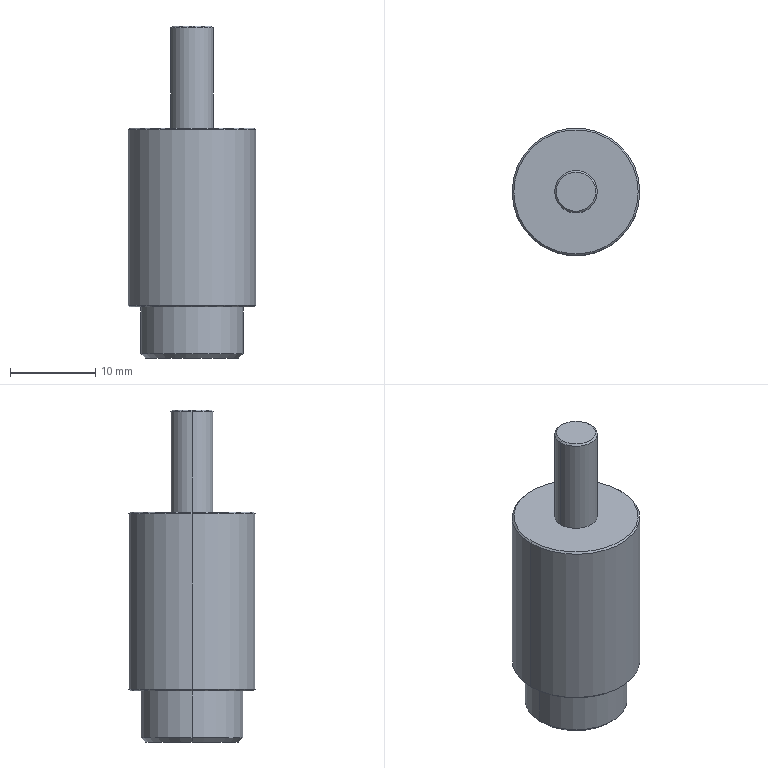Part | SolidWorks | features Chamfer 3, ICE 2, Extrusion 1 | 1 solid | 18 faces | box 15 x 15 x 39 mm | volume 4618 mm3 | cone 8 | cylinder 6 | plane 4 | commonest cylinder face diameters 5 x2 12 x2 15 x2
STEP:
#1=CARTESIAN_POINT('',(7.3,0.,13.5));
#2=VERTEX_POINT('',#1);
#3=CARTESIAN_POINT('',(-7.3,0.,13.5));
#4=VERTEX_POINT('',#3);
#5=CARTESIAN_POINT('',(0.,0.,13.5));
#6=DIRECTION('',(0.,0.,1.));
#7=DIRECTION('',(1.,0.,0.));
#8=AXIS2_PLACEMENT_3D('',#5,#6,#7);
#9=CIRCLE('',#8,7.3);
#10=EDGE_CURVE('',#2,#4,#9,.T.);
#11=ORIENTED_EDGE('',*,*,#10,.F.);
#12=CARTESIAN_POINT('',(7.5,0.,13.3));
#13=VERTEX_POINT('',#12);
#14=CARTESIAN_POINT('',(7.3,0.,13.5));
#15=DIRECTION('',(0.7071,0.,-0.7071));
#16=VECTOR('',#15,1000.);
#17=LINE('',#14,#16);
#18=EDGE_CURVE('',#2,#13,#17,.T.);
#19=ORIENTED_EDGE('',*,*,#18,.T.);
#20=CARTESIAN_POINT('',(-7.5,0.,13.3));
#21=VERTEX_POINT('',#20);
#22=CARTESIAN_POINT('',(0.,0.,13.3));
#23=DIRECTION('',(0.,0.,-1.));
#24=DIRECTION('',(1.,0.,0.));
#25=AXIS2_PLACEMENT_3D('',#22,#23,#24);
#26=CIRCLE('',#25,7.5);
#27=EDGE_CURVE('',#21,#13,#26,.T.);
#28=ORIENTED_EDGE('',*,*,#27,.F.);
#29=CARTESIAN_POINT('',(-7.3,0.,13.5));
#30=DIRECTION('',(-0.7071,0.,-0.7071));
#31=VECTOR('',#30,1000.);
#32=LINE('',#29,#31);
#33=EDGE_CURVE('',#4,#21,#32,.T.);
#34=ORIENTED_EDGE('',*,*,#33,.F.);
#35=EDGE_LOOP('',(#11,#19,#28,#34));
#36=FACE_OUTER_BOUND('',#35,.T.);
#37=CARTESIAN_POINT('',(0.,0.,13.5));
#38=DIRECTION('',(0.,0.,-1.));
#39=DIRECTION('',(-1.,0.,0.));
#40=AXIS2_PLACEMENT_3D('',#37,#38,#39);
#41=CONICAL_SURFACE('',#40,7.3,0.7854);
#42=ADVANCED_FACE('',(#36),#41,.T.);
#43=CARTESIAN_POINT('',(-7.3,0.,-7.5));
#44=VERTEX_POINT('',#43);
#45=CARTESIAN_POINT('',(7.3,0.,-7.5));
#46=VERTEX_POINT('',#45);
#47=CARTESIAN_POINT('',(0.,0.,-7.5));
#48=DIRECTION('',(0.,0.,-1.));
#49=DIRECTION('',(1.,0.,0.));
#50=AXIS2_PLACEMENT_3D('',#47,#48,#49);
#51=CIRCLE('',#50,7.3);
#52=EDGE_CURVE('',#44,#46,#51,.T.);
#53=ORIENTED_EDGE('',*,*,#52,.F.);
#54=CARTESIAN_POINT('',(-7.5,0.,-7.3));
#55=VERTEX_POINT('',#54);
#56=CARTESIAN_POINT('',(-7.5,0.,-7.3));
#57=DIRECTION('',(-0.7071,0.,0.7071));
#58=VECTOR('',#57,1000.);
#59=LINE('',#56,#58);
#60=EDGE_CURVE('',#44,#55,#59,.T.);
#61=ORIENTED_EDGE('',*,*,#60,.T.);
#62=CARTESIAN_POINT('',(7.5,0.,-7.3));
#63=VERTEX_POINT('',#62);
#64=CARTESIAN_POINT('',(0.,0.,-7.3));
#65=DIRECTION('',(0.,0.,1.));
#66=DIRECTION('',(1.,0.,0.));
#67=AXIS2_PLACEMENT_3D('',#64,#65,#66);
#68=CIRCLE('',#67,7.5);
#69=EDGE_CURVE('',#63,#55,#68,.T.);
#70=ORIENTED_EDGE('',*,*,#69,.F.);
#71=CARTESIAN_POINT('',(7.5,0.,-7.3));
#72=DIRECTION('',(0.7071,0.,0.7071));
#73=VECTOR('',#72,1000.);
#74=LINE('',#71,#73);
#75=EDGE_CURVE('',#46,#63,#74,.T.);
#76=ORIENTED_EDGE('',*,*,#75,.F.);
#77=EDGE_LOOP('',(#53,#61,#70,#76));
#78=FACE_OUTER_BOUND('',#77,.T.);
#79=CARTESIAN_POINT('',(0.,0.,-7.3));
#80=DIRECTION('',(0.,0.,1.));
#81=DIRECTION('',(1.,0.,0.));
#82=AXIS2_PLACEMENT_3D('',#79,#80,#81);
#83=CONICAL_SURFACE('',#82,7.5,0.7854);
#84=ADVANCED_FACE('',(#78),#83,.T.);
#85=CARTESIAN_POINT('',(6.,0.,-7.5));
#86=VERTEX_POINT('',#85);
#87=CARTESIAN_POINT('',(-6.,0.,-7.5));
#88=VERTEX_POINT('',#87);
#89=CARTESIAN_POINT('',(0.,0.,-7.5));
#90=DIRECTION('',(0.,0.,1.));
#91=DIRECTION('',(1.,0.,0.));
#92=AXIS2_PLACEMENT_3D('',#89,#90,#91);
#93=CIRCLE('',#92,6.);
#94=EDGE_CURVE('',#86,#88,#93,.T.);
#95=ORIENTED_EDGE('',*,*,#94,.F.);
#96=CARTESIAN_POINT('',(6.,0.,-13.));
#97=VERTEX_POINT('',#96);
#98=CARTESIAN_POINT('',(6.,0.,13.5));
#99=DIRECTION('',(0.,0.,-1.));
#100=VECTOR('',#99,1000.);
#101=LINE('',#98,#100);
#102=EDGE_CURVE('',#86,#97,#101,.T.);
#103=ORIENTED_EDGE('',*,*,#102,.T.);
#104=CARTESIAN_POINT('',(-6.,0.,-13.));
#105=VERTEX_POINT('',#104);
#106=CARTESIAN_POINT('',(0.,0.,-13.));
#107=DIRECTION('',(0.,0.,1.));
#108=DIRECTION('',(1.,0.,0.));
#109=AXIS2_PLACEMENT_3D('',#106,#107,#108);
#110=CIRCLE('',#109,6.);
#111=EDGE_CURVE('',#97,#105,#110,.T.);
#112=ORIENTED_EDGE('',*,*,#111,.T.);
#113=CARTESIAN_POINT('',(-6.,0.,13.5));
#114=DIRECTION('',(0.,0.,-1.));
#115=VECTOR('',#114,1000.);
#116=LINE('',#113,#115);
#117=EDGE_CURVE('',#88,#105,#116,.T.);
#118=ORIENTED_EDGE('',*,*,#117,.F.);
#119=EDGE_LOOP('',(#95,#103,#112,#118));
#120=FACE_OUTER_BOUND('',#119,.T.);
#121=CARTESIAN_POINT('',(0.,0.,13.5));
#122=DIRECTION('',(0.,0.,-1.));
#123=DIRECTION('',(-1.,0.,0.));
#124=AXIS2_PLACEMENT_3D('',#121,#122,#123);
#125=CYLINDRICAL_SURFACE('',#124,6.);
#126=ADVANCED_FACE('',(#120),#125,.T.);
#127=CARTESIAN_POINT('',(-5.5,0.,-13.5));
#128=VERTEX_POINT('',#127);
#129=CARTESIAN_POINT('',(5.5,0.,-13.5));
#130=VERTEX_POINT('',#129);
#131=CARTESIAN_POINT('',(0.,0.,-13.5));
#132=DIRECTION('',(0.,0.,-1.));
#133=DIRECTION('',(1.,0.,0.));
#134=AXIS2_PLACEMENT_3D('',#131,#132,#133);
#135=CIRCLE('',#134,5.5);
#136=EDGE_CURVE('',#128,#130,#135,.T.);
#137=ORIENTED_EDGE('',*,*,#136,.F.);
#138=CARTESIAN_POINT('',(-6.,0.,-13.));
#139=DIRECTION('',(-0.7071,0.,0.7071));
#140=VECTOR('',#139,1000.);
#141=LINE('',#138,#140);
#142=EDGE_CURVE('',#128,#105,#141,.T.);
#143=ORIENTED_EDGE('',*,*,#142,.T.);
#144=ORIENTED_EDGE('',*,*,#111,.F.);
#145=CARTESIAN_POINT('',(6.,0.,-13.));
#146=DIRECTION('',(0.7071,0.,0.7071));
#147=VECTOR('',#146,1000.);
#148=LINE('',#145,#147);
#149=EDGE_CURVE('',#130,#97,#148,.T.);
#150=ORIENTED_EDGE('',*,*,#149,.F.);
#151=EDGE_LOOP('',(#137,#143,#144,#150));
#152=FACE_OUTER_BOUND('',#151,.T.);
#153=CARTESIAN_POINT('',(0.,0.,-13.));
#154=DIRECTION('',(0.,0.,1.));
#155=DIRECTION('',(1.,0.,0.));
#156=AXIS2_PLACEMENT_3D('',#153,#154,#155);
#157=CONICAL_SURFACE('',#156,6.,0.7854);
#158=ADVANCED_FACE('',(#152),#157,.T.);
#159=ORIENTED_EDGE('',*,*,#69,.T.);
#160=CARTESIAN_POINT('',(-7.5,0.,-7.5));
#161=DIRECTION('',(0.,0.,1.));
#162=VECTOR('',#161,1000.);
#163=LINE('',#160,#162);
#164=EDGE_CURVE('',#55,#21,#163,.T.);
#165=ORIENTED_EDGE('',*,*,#164,.T.);
#166=ORIENTED_EDGE('',*,*,#27,.T.);
#167=CARTESIAN_POINT('',(7.5,0.,-7.5));
#168=DIRECTION('',(0.,0.,1.));
#169=VECTOR('',#168,1000.);
#170=LINE('',#167,#169);
#171=EDGE_CURVE('',#63,#13,#170,.T.);
#172=ORIENTED_EDGE('',*,*,#171,.F.);
#173=EDGE_LOOP('',(#159,#165,#166,#172));
#174=FACE_OUTER_BOUND('',#173,.T.);
#175=CARTESIAN_POINT('',(0.,0.,-7.5));
#176=DIRECTION('',(0.,0.,1.));
#177=DIRECTION('',(1.,0.,0.));
#178=AXIS2_PLACEMENT_3D('',#175,#176,#177);
#179=CYLINDRICAL_SURFACE('',#178,7.5);
#180=ADVANCED_FACE('',(#174),#179,.T.);
#181=CARTESIAN_POINT('',(2.3,0.,25.5));
#182=VERTEX_POINT('',#181);
#183=CARTESIAN_POINT('',(-2.3,0.,25.5));
#184=VERTEX_POINT('',#183);
#185=CARTESIAN_POINT('',(0.,0.,25.5));
#186=DIRECTION('',(0.,0.,1.));
#187=DIRECTION('',(1.,0.,0.));
#188=AXIS2_PLACEMENT_3D('',#185,#186,#187);
#189=CIRCLE('',#188,2.3);
#190=EDGE_CURVE('',#182,#184,#189,.T.);
#191=ORIENTED_EDGE('',*,*,#190,.F.);
#192=CARTESIAN_POINT('',(2.5,0.,25.3));
#193=VERTEX_POINT('',#192);
#194=CARTESIAN_POINT('',(2.3,0.,25.5));
#195=DIRECTION('',(0.7071,0.,-0.7071));
#196=VECTOR('',#195,1000.);
#197=LINE('',#194,#196);
#198=EDGE_CURVE('',#182,#193,#197,.T.);
#199=ORIENTED_EDGE('',*,*,#198,.T.);
#200=CARTESIAN_POINT('',(-2.5,0.,25.3));
#201=VERTEX_POINT('',#200);
#202=CARTESIAN_POINT('',(0.,0.,25.3));
#203=DIRECTION('',(0.,0.,-1.));
#204=DIRECTION('',(1.,0.,0.));
#205=AXIS2_PLACEMENT_3D('',#202,#203,#204);
#206=CIRCLE('',#205,2.5);
#207=EDGE_CURVE('',#201,#193,#206,.T.);
#208=ORIENTED_EDGE('',*,*,#207,.F.);
#209=CARTESIAN_POINT('',(-2.3,0.,25.5));
#210=DIRECTION('',(-0.7071,0.,-0.7071));
#211=VECTOR('',#210,1000.);
#212=LINE('',#209,#211);
#213=EDGE_CURVE('',#184,#201,#212,.T.);
#214=ORIENTED_EDGE('',*,*,#213,.F.);
#215=EDGE_LOOP('',(#191,#199,#208,#214));
#216=FACE_OUTER_BOUND('',#215,.T.);
#217=CARTESIAN_POINT('',(0.,0.,25.5));
#218=DIRECTION('',(0.,0.,-1.));
#219=DIRECTION('',(-1.,0.,0.));
#220=AXIS2_PLACEMENT_3D('',#217,#218,#219);
#221=CONICAL_SURFACE('',#220,2.3,0.7854);
#222=ADVANCED_FACE('',(#216),#221,.T.);
#223=ORIENTED_EDGE('',*,*,#207,.T.);
#224=CARTESIAN_POINT('',(2.5,0.,13.5));
#225=VERTEX_POINT('',#224);
#226=CARTESIAN_POINT('',(2.5,0.,25.5));
#227=DIRECTION('',(0.,0.,-1.));
#228=VECTOR('',#227,1000.);
#229=LINE('',#226,#228);
#230=EDGE_CURVE('',#193,#225,#229,.T.);
#231=ORIENTED_EDGE('',*,*,#230,.T.);
#232=CARTESIAN_POINT('',(-2.5,0.,13.5));
#233=VERTEX_POINT('',#232);
#234=CARTESIAN_POINT('',(0.,0.,13.5));
#235=DIRECTION('',(0.,0.,1.));
#236=DIRECTION('',(1.,0.,0.));
#237=AXIS2_PLACEMENT_3D('',#234,#235,#236);
#238=CIRCLE('',#237,2.5);
#239=EDGE_CURVE('',#225,#233,#238,.T.);
#240=ORIENTED_EDGE('',*,*,#239,.T.);
#241=CARTESIAN_POINT('',(-2.5,0.,25.5));
#242=DIRECTION('',(0.,0.,-1.));
#243=VECTOR('',#242,1000.);
#244=LINE('',#241,#243);
#245=EDGE_CURVE('',#201,#233,#244,.T.);
#246=ORIENTED_EDGE('',*,*,#245,.F.);
#247=EDGE_LOOP('',(#223,#231,#240,#246));
#248=FACE_OUTER_BOUND('',#247,.T.);
#249=CARTESIAN_POINT('',(0.,0.,25.5));
#250=DIRECTION('',(0.,0.,-1.));
#251=DIRECTION('',(-1.,0.,0.));
#252=AXIS2_PLACEMENT_3D('',#249,#250,#251);
#253=CYLINDRICAL_SURFACE('',#252,2.5);
#254=ADVANCED_FACE('',(#248),#253,.T.);
#255=CARTESIAN_POINT('',(0.,0.,13.5));
#256=DIRECTION('',(0.,0.,1.));
#257=DIRECTION('',(1.,0.,0.));
#258=AXIS2_PLACEMENT_3D('',#255,#256,#257);
#259=CIRCLE('',#258,7.3);
#260=EDGE_CURVE('',#4,#2,#259,.T.);
#261=ORIENTED_EDGE('',*,*,#260,.T.);
#262=ORIENTED_EDGE('',*,*,#10,.T.);
#263=EDGE_LOOP('',(#261,#262));
#264=FACE_OUTER_BOUND('',#263,.T.);
#265=CARTESIAN_POINT('',(0.,0.,13.5));
#266=DIRECTION('',(0.,0.,1.));
#267=DIRECTION('',(1.,0.,0.));
#268=AXIS2_PLACEMENT_3D('',#265,#266,#267);
#269=CIRCLE('',#268,2.5);
#270=EDGE_CURVE('',#233,#225,#269,.T.);
#271=ORIENTED_EDGE('',*,*,#270,.F.);
#272=ORIENTED_EDGE('',*,*,#239,.F.);
#273=EDGE_LOOP('',(#271,#272));
#274=FACE_BOUND('',#273,.T.);
#275=CARTESIAN_POINT('',(0.,0.,13.5));
#276=DIRECTION('',(0.,0.,1.));
#277=DIRECTION('',(1.,0.,0.));
#278=AXIS2_PLACEMENT_3D('',#275,#276,#277);
#279=PLANE('',#278);
#280=ADVANCED_FACE('',(#264,#274),#279,.T.);
#281=ORIENTED_EDGE('',*,*,#230,.F.);
#282=CARTESIAN_POINT('',(0.,0.,25.3));
#283=DIRECTION('',(0.,0.,-1.));
#284=DIRECTION('',(1.,0.,0.));
#285=AXIS2_PLACEMENT_3D('',#282,#283,#284);
#286=CIRCLE('',#285,2.5);
#287=EDGE_CURVE('',#193,#201,#286,.T.);
#288=ORIENTED_EDGE('',*,*,#287,.T.);
#289=ORIENTED_EDGE('',*,*,#245,.T.);
#290=ORIENTED_EDGE('',*,*,#270,.T.);
#291=EDGE_LOOP('',(#281,#288,#289,#290));
#292=FACE_OUTER_BOUND('',#291,.T.);
#293=CARTESIAN_POINT('',(0.,0.,25.5));
#294=DIRECTION('',(0.,0.,-1.));
#295=DIRECTION('',(-1.,0.,0.));
#296=AXIS2_PLACEMENT_3D('',#293,#294,#295);
#297=CYLINDRICAL_SURFACE('',#296,2.5);
#298=ADVANCED_FACE('',(#292),#297,.T.);
#299=CARTESIAN_POINT('',(0.,0.,25.5));
#300=DIRECTION('',(0.,0.,1.));
#301=DIRECTION('',(1.,0.,0.));
#302=AXIS2_PLACEMENT_3D('',#299,#300,#301);
#303=CIRCLE('',#302,2.3);
#304=EDGE_CURVE('',#184,#182,#303,.T.);
#305=ORIENTED_EDGE('',*,*,#304,.T.);
#306=ORIENTED_EDGE('',*,*,#190,.T.);
#307=EDGE_LOOP('',(#305,#306));
#308=FACE_OUTER_BOUND('',#307,.T.);
#309=CARTESIAN_POINT('',(0.,0.,25.5));
#310=DIRECTION('',(0.,0.,1.));
#311=DIRECTION('',(1.,0.,0.));
#312=AXIS2_PLACEMENT_3D('',#309,#310,#311);
#313=PLANE('',#312);
#314=ADVANCED_FACE('',(#308),#313,.T.);
#315=ORIENTED_EDGE('',*,*,#198,.F.);
#316=ORIENTED_EDGE('',*,*,#304,.F.);
#317=ORIENTED_EDGE('',*,*,#213,.T.);
#318=ORIENTED_EDGE('',*,*,#287,.F.);
#319=EDGE_LOOP('',(#315,#316,#317,#318));
#320=FACE_OUTER_BOUND('',#319,.T.);
#321=CARTESIAN_POINT('',(0.,0.,25.5));
#322=DIRECTION('',(0.,0.,-1.));
#323=DIRECTION('',(-1.,0.,0.));
#324=AXIS2_PLACEMENT_3D('',#321,#322,#323);
#325=CONICAL_SURFACE('',#324,2.3,0.7854);
#326=ADVANCED_FACE('',(#320),#325,.T.);
#327=CARTESIAN_POINT('',(0.,0.,-7.5));
#328=DIRECTION('',(0.,0.,-1.));
#329=DIRECTION('',(1.,0.,0.));
#330=AXIS2_PLACEMENT_3D('',#327,#328,#329);
#331=CIRCLE('',#330,7.3);
#332=EDGE_CURVE('',#46,#44,#331,.T.);
#333=ORIENTED_EDGE('',*,*,#332,.T.);
#334=ORIENTED_EDGE('',*,*,#52,.T.);
#335=EDGE_LOOP('',(#333,#334));
#336=FACE_OUTER_BOUND('',#335,.T.);
#337=CARTESIAN_POINT('',(0.,0.,-7.5));
#338=DIRECTION('',(0.,0.,1.));
#339=DIRECTION('',(1.,0.,0.));
#340=AXIS2_PLACEMENT_3D('',#337,#338,#339);
#341=CIRCLE('',#340,6.);
#342=EDGE_CURVE('',#88,#86,#341,.T.);
#343=ORIENTED_EDGE('',*,*,#342,.T.);
#344=ORIENTED_EDGE('',*,*,#94,.T.);
#345=EDGE_LOOP('',(#343,#344));
#346=FACE_BOUND('',#345,.T.);
#347=CARTESIAN_POINT('',(0.,0.,-7.5));
#348=DIRECTION('',(0.,0.,1.));
#349=DIRECTION('',(1.,0.,0.));
#350=AXIS2_PLACEMENT_3D('',#347,#348,#349);
#351=PLANE('',#350);
#352=ADVANCED_FACE('',(#336,#346),#351,.F.);
#353=ORIENTED_EDGE('',*,*,#164,.F.);
#354=CARTESIAN_POINT('',(0.,0.,-7.3));
#355=DIRECTION('',(0.,0.,1.));
#356=DIRECTION('',(1.,0.,0.));
#357=AXIS2_PLACEMENT_3D('',#354,#355,#356);
#358=CIRCLE('',#357,7.5);
#359=EDGE_CURVE('',#55,#63,#358,.T.);
#360=ORIENTED_EDGE('',*,*,#359,.T.);
#361=ORIENTED_EDGE('',*,*,#171,.T.);
#362=CARTESIAN_POINT('',(0.,0.,13.3));
#363=DIRECTION('',(0.,0.,-1.));
#364=DIRECTION('',(1.,0.,0.));
#365=AXIS2_PLACEMENT_3D('',#362,#363,#364);
#366=CIRCLE('',#365,7.5);
#367=EDGE_CURVE('',#13,#21,#366,.T.);
#368=ORIENTED_EDGE('',*,*,#367,.T.);
#369=EDGE_LOOP('',(#353,#360,#361,#368));
#370=FACE_OUTER_BOUND('',#369,.T.);
#371=CARTESIAN_POINT('',(0.,0.,-7.5));
#372=DIRECTION('',(0.,0.,1.));
#373=DIRECTION('',(1.,0.,0.));
#374=AXIS2_PLACEMENT_3D('',#371,#372,#373);
#375=CYLINDRICAL_SURFACE('',#374,7.5);
#376=ADVANCED_FACE('',(#370),#375,.T.);
#377=CARTESIAN_POINT('',(0.,0.,-13.5));
#378=DIRECTION('',(0.,0.,-1.));
#379=DIRECTION('',(1.,0.,0.));
#380=AXIS2_PLACEMENT_3D('',#377,#378,#379);
#381=CIRCLE('',#380,5.5);
#382=EDGE_CURVE('',#130,#128,#381,.T.);
#383=ORIENTED_EDGE('',*,*,#382,.T.);
#384=ORIENTED_EDGE('',*,*,#136,.T.);
#385=EDGE_LOOP('',(#383,#384));
#386=FACE_OUTER_BOUND('',#385,.T.);
#387=CARTESIAN_POINT('',(0.,0.,-13.5));
#388=DIRECTION('',(0.,0.,1.));
#389=DIRECTION('',(1.,0.,0.));
#390=AXIS2_PLACEMENT_3D('',#387,#388,#389);
#391=PLANE('',#390);
#392=ADVANCED_FACE('',(#386),#391,.F.);
#393=ORIENTED_EDGE('',*,*,#142,.F.);
#394=ORIENTED_EDGE('',*,*,#382,.F.);
#395=ORIENTED_EDGE('',*,*,#149,.T.);
#396=CARTESIAN_POINT('',(0.,0.,-13.));
#397=DIRECTION('',(0.,0.,1.));
#398=DIRECTION('',(1.,0.,0.));
#399=AXIS2_PLACEMENT_3D('',#396,#397,#398);
#400=CIRCLE('',#399,6.);
#401=EDGE_CURVE('',#105,#97,#400,.T.);
#402=ORIENTED_EDGE('',*,*,#401,.F.);
#403=EDGE_LOOP('',(#393,#394,#395,#402));
#404=FACE_OUTER_BOUND('',#403,.T.);
#405=CARTESIAN_POINT('',(0.,0.,-13.));
#406=DIRECTION('',(0.,0.,1.));
#407=DIRECTION('',(1.,0.,0.));
#408=AXIS2_PLACEMENT_3D('',#405,#406,#407);
#409=CONICAL_SURFACE('',#408,6.,0.7854);
#410=ADVANCED_FACE('',(#404),#409,.T.);
#411=ORIENTED_EDGE('',*,*,#102,.F.);
#412=ORIENTED_EDGE('',*,*,#342,.F.);
#413=ORIENTED_EDGE('',*,*,#117,.T.);
#414=ORIENTED_EDGE('',*,*,#401,.T.);
#415=EDGE_LOOP('',(#411,#412,#413,#414));
#416=FACE_OUTER_BOUND('',#415,.T.);
#417=CARTESIAN_POINT('',(0.,0.,13.5));
#418=DIRECTION('',(0.,0.,-1.));
#419=DIRECTION('',(-1.,0.,0.));
#420=AXIS2_PLACEMENT_3D('',#417,#418,#419);
#421=CYLINDRICAL_SURFACE('',#420,6.);
#422=ADVANCED_FACE('',(#416),#421,.T.);
#423=ORIENTED_EDGE('',*,*,#60,.F.);
#424=ORIENTED_EDGE('',*,*,#332,.F.);
#425=ORIENTED_EDGE('',*,*,#75,.T.);
#426=ORIENTED_EDGE('',*,*,#359,.F.);
#427=EDGE_LOOP('',(#423,#424,#425,#426));
#428=FACE_OUTER_BOUND('',#427,.T.);
#429=CARTESIAN_POINT('',(0.,0.,-7.3));
#430=DIRECTION('',(0.,0.,1.));
#431=DIRECTION('',(1.,0.,0.));
#432=AXIS2_PLACEMENT_3D('',#429,#430,#431);
#433=CONICAL_SURFACE('',#432,7.5,0.7854);
#434=ADVANCED_FACE('',(#428),#433,.T.);
#435=ORIENTED_EDGE('',*,*,#18,.F.);
#436=ORIENTED_EDGE('',*,*,#260,.F.);
#437=ORIENTED_EDGE('',*,*,#33,.T.);
#438=ORIENTED_EDGE('',*,*,#367,.F.);
#439=EDGE_LOOP('',(#435,#436,#437,#438));
#440=FACE_OUTER_BOUND('',#439,.T.);
#441=CARTESIAN_POINT('',(0.,0.,13.5));
#442=DIRECTION('',(0.,0.,-1.));
#443=DIRECTION('',(-1.,0.,0.));
#444=AXIS2_PLACEMENT_3D('',#441,#442,#443);
#445=CONICAL_SURFACE('',#444,7.3,0.7854);
#446=ADVANCED_FACE('',(#440),#445,.T.);
#447=CLOSED_SHELL('',(#42,#84,#126,#158,#180,#222,#254,#280,#298,#314,#326,#352,#376,#392,#410,#422,#434,#446));
#448=MANIFOLD_SOLID_BREP('',#447);
#449=CARTESIAN_POINT('',(0.,0.,0.));
#450=DIRECTION('',(0.,0.,1.));
#451=DIRECTION('',(1.,0.,0.));
#452=AXIS2_PLACEMENT_3D('',#449,#450,#451);
#453=(LENGTH_UNIT()NAMED_UNIT(*)SI_UNIT(.MILLI.,.METRE.));
#454=UNCERTAINTY_MEASURE_WITH_UNIT(LENGTH_MEASURE(0.00001),#453,'','');
#455=(NAMED_UNIT(*)PLANE_ANGLE_UNIT()SI_UNIT($,.RADIAN.));
#456=(NAMED_UNIT(*)SI_UNIT($,.STERADIAN.)SOLID_ANGLE_UNIT());
#457=(GEOMETRIC_REPRESENTATION_CONTEXT(3)GLOBAL_UNCERTAINTY_ASSIGNED_CONTEXT((#454))GLOBAL_UNIT_ASSIGNED_CONTEXT((#453,#455,#456))REPRESENTATION_CONTEXT('',''));
#458=ADVANCED_BREP_SHAPE_REPRESENTATION('',(#448,#452),#457);